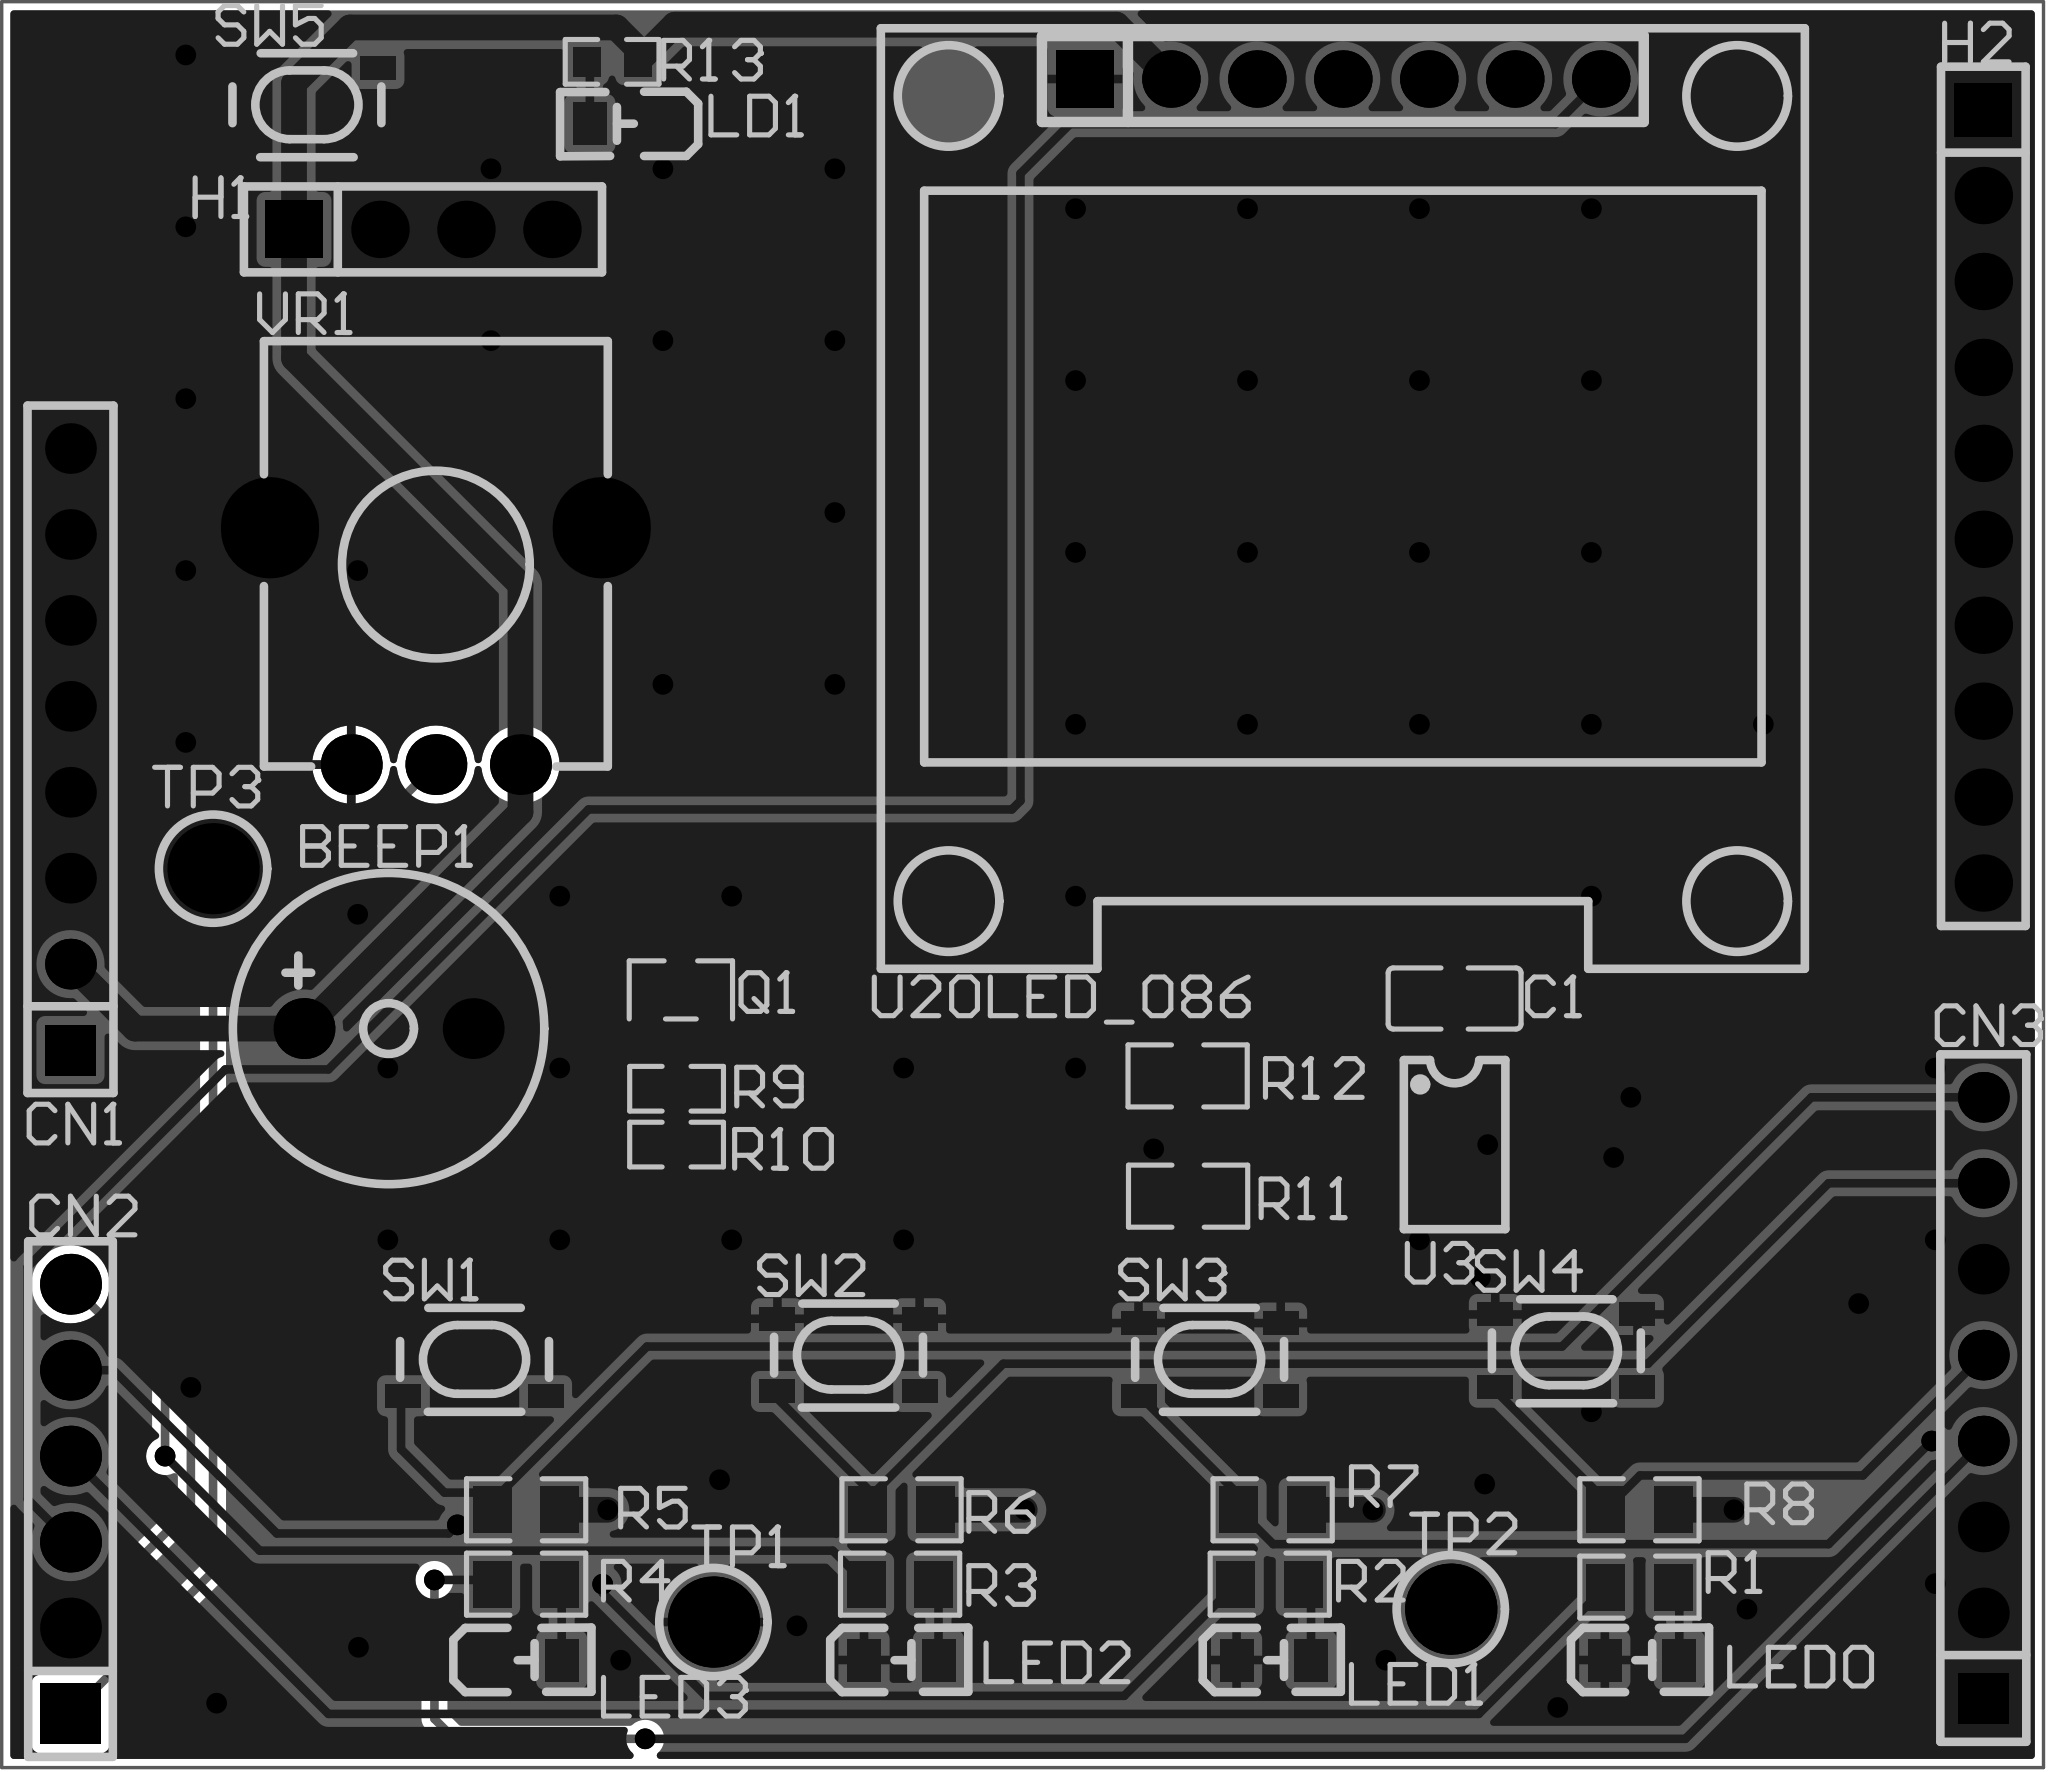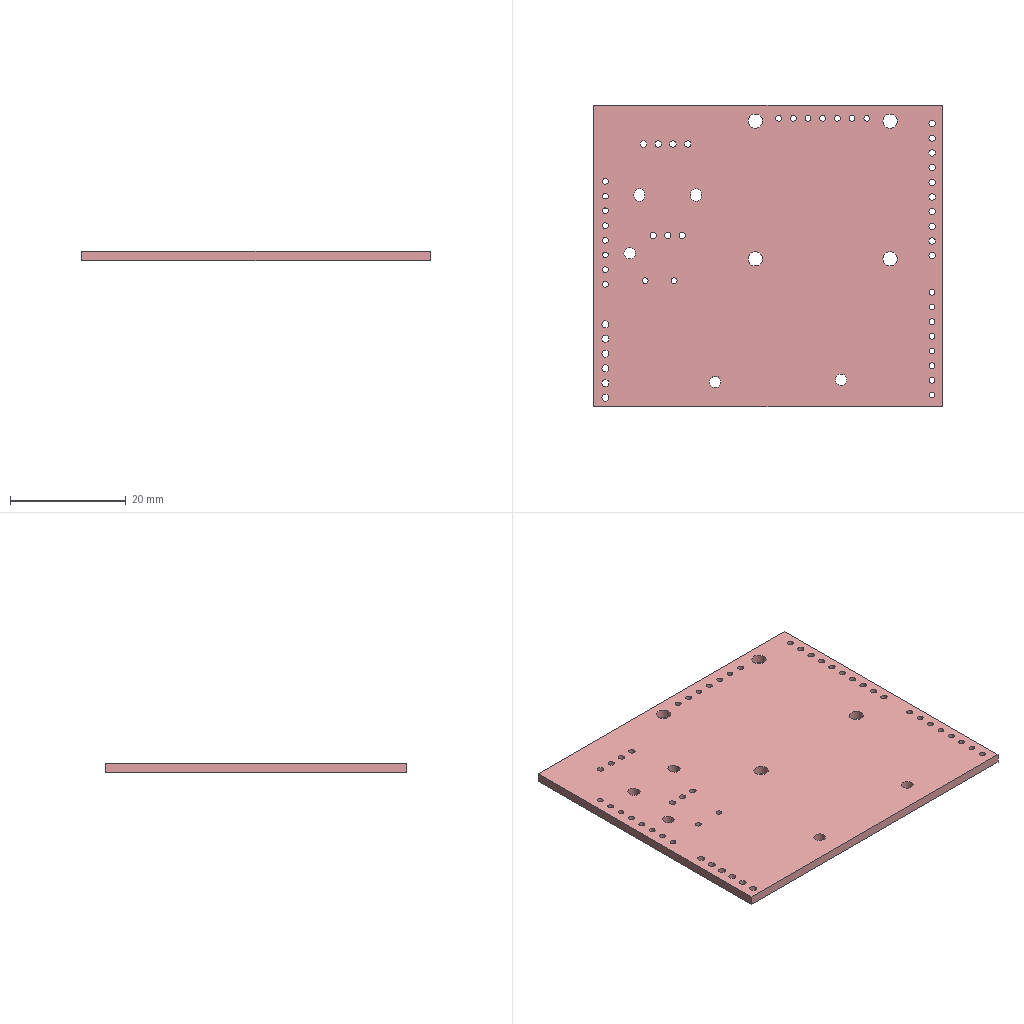Circuit board layout | Altium Designer | box 60.3 x 52.2 x 1.6 mm
Layer stack:
# Altium Designer layer stack of  (unit mm; dielectric type: 0 none, 1 core, 2 prepreg, 3 surface material)
index,name,kind,layer,copper_thickness_mm,dielectric_type,dielectric_thickness_mm,dielectric_material,dielectric_constant
0,Top Paste Mask Layer,other,,,,,,
1,Top Silkscreen Layer,other,,,,,,
2,Top Solder Mask Layer,dielectric,,,3,0.01,,3.3
3,Top Layer,copper,Top Layer,0.035,,,,
4,Dielectric1,dielectric,,,3,1.51,FR4,4.5
5,Bottom Layer,copper,Bottom Layer,0.035,,,,
6,Bottom Solder Mask Layer,dielectric,,,3,0.01,,3.3
7,Bottom Silkscreen Layer,other,,,,,,
8,Bottom Paste Mask Layer,other,,,,,,
# drill layer pairs: low layer,high layer
drill_pair,Top Layer,Bottom Layer
Part placement:
Designator,Comment,Layer,Footprint,Center-X(mm),Center-Y(mm),Rotation
BEEP1,3kHz,TopLayer,BUZ-TH_BD9.0-P5.00-D0.6-FD,96.139,112.014,0
C1,100nF,TopLayer,C0805,127.635,112.903,180
CN1,,TopLayer,HDR-TH_8P-P2.54-V-M,86.741,120.269,90
CN2,,TopLayer,HDR-TH_6P-P2.54-V-M-1,86.742,98.106,90
CN3,,TopLayer,HDR-TH_8P-P2.54-V-M,143.256,101.092,90
H1,,TopLayer,HDR-TH_4P-P2.54-V-F,97.155,135.636,0
H2,,TopLayer,HDR-TH_10P-P2.54-V-M-1,143.256,127.746,270
LD1,NCD0805R1,TopLayer,LED0805-RD,103.186,138.756,180
LED0,,TopLayer,LED_0805,133.173,93.35,0
LED1,,TopLayer,LED_0805,122.293,93.35,0
LED2,,TopLayer,LED_0805,111.287,93.35,0
LED3,,TopLayer,LED_0805,100.153,93.35,0
Q1,S8050 J3Y(RANGE:200-350),TopLayer,SOT-23-3_L3.0-W1.7-P0.95-LS2.9-BR,104.775,113.157,270
R1,4.7K,TopLayer,R0805,133.096,95.504,0
R2,4.7K,TopLayer,R0805,122.174,95.592,0
R3,4.7K,TopLayer,R0805,111.252,95.592,0
R4,4.7K,TopLayer,R0805,100.203,95.592,0
R5,4.7kΩ,TopLayer,R0805,100.203,97.79,0
R6,4.7kΩ,TopLayer,R0805,111.294,97.79,0
R7,4.7kΩ,TopLayer,R0805,122.259,97.79,0
R8,4.7kΩ,TopLayer,R0805,133.096,97.79,0
R9,1K,TopLayer,R0603,104.648,110.236,0
R10,10K,TopLayer,R0603,104.648,108.585,180
R11,4.7kΩ,TopLayer,R0805,119.761,107.061,180
R12,4.7kΩ,TopLayer,R0805,119.747,110.615,0
R13,4.7K,TopLayer,R0603,102.743,140.589,0
TP1,TP-红色测试点,TopLayer,TESTPOINT-TH_BD3.2,105.736,94.472,0
TP2,TP-红色测试点,TopLayer,TESTPOINT-TH_BD3.2,127.521,94.853,0
TP3,TP-红色测试点,TopLayer,TESTPOINT-TH_BD3.2,90.953,116.74,0
U2OLED_086,0.96寸OLED_7P,TopLayer,OLED-TH_HS96L01W4S03,124.333,140.081,0
U3,LM75AD,118,TopLayer,SOIC-8_L5.0-W4.0-P1.27-LS6.0-BL,127.635,108.585,270
VR1,10kΩ,TopLayer,RES-ADJ-TH_RK09K1130AJ3,97.536,123.317,0
SW1,,TopLayer,Key_SMD_4.2x3.2x2.5,98.679,102.235,0
SW2,,TopLayer,Key_SMD_4.2x3.2x2.5,109.728,102.362,0
SW3,,TopLayer,Key_SMD_4.2x3.2x2.5,120.396,102.235,0
SW4,,TopLayer,Key_SMD_4.2x3.2x2.5,130.937,102.489,0
SW5,,TopLayer,Key_SMD_4.2x3.2x2.5,93.726,139.319,0
Pad and via stacks:
# Altium Designer via and pad stacks of  (unit mm). Each distinct definition once, with the count of objects using it.
# via: kind,start_layer,end_layer,hole_mm,diameter_mm,mode(0 simple;1 top-mid-bottom;2 full stack),diameter_per_layer,count,example_net
# pad: kind,layer,hole_mm,hole_type(0 round;1 square;2 slot),plating,top_size,top_shape(1 round;2 rect;3 octagon;9 rounded rect),mid_size,bottom_size,mode,footprint,size_per_layer,count,example
pad,Multi-Layer,1,0,plated,1.8x1.8,1,1.8x1.8,1.8x1.8,0,BUZ-TH_BD9.0-P5.00-D0.6-FD,,2,BEEP1.1
pad,Multi-Layer,1,0,plated,1.5x1.5,2,1.5x1.5,1.5x1.5,0,HDR-TH_8P-P2.54-V-M,,2,CN1.1
pad,Multi-Layer,1,0,plated,1.5x1.5,1,1.5x1.5,1.5x1.5,0,HDR-TH_8P-P2.54-V-M,,14,CN1.2
pad,Multi-Layer,1.2,0,plated,1.8x1.8,1,1.8x1.8,1.8x1.8,0,HDR-TH_6P-P2.54-V-M-1,,5,CN2.6
pad,Multi-Layer,1.2,0,plated,1.8x1.8,2,1.8x1.8,1.8x1.8,0,HDR-TH_6P-P2.54-V-M-1,,1,CN2.1
pad,Multi-Layer,1.1,0,plated,1.7x1.7,2,1.7x1.7,1.7x1.7,0,HDR-TH_4P-P2.54-V-F,,1,H1.1
pad,Multi-Layer,1.1,0,plated,1.7x1.7,1,1.7x1.7,1.7x1.7,0,HDR-TH_4P-P2.54-V-F,,3,H1.2
pad,Multi-Layer,1.1,0,plated,1.7x1.7,1,1.7x1.7,1.7x1.7,0,HDR-TH_10P-P2.54-V-M-1,,9,H2.10
pad,Multi-Layer,1.1,0,plated,1.575x1.7,2,1.575x1.7,1.575x1.7,0,HDR-TH_10P-P2.54-V-M-1,,1,H2.1
pad,Multi-Layer,2,0,plated,2.7x2.7,1,2.7x2.7,2.7x2.7,0,TESTPOINT-TH_BD3.2,,3,TP1.1
pad,Multi-Layer,1,0,plated,1.7x1.7,1,1.7x1.7,1.7x1.7,0,OLED-TH_HS96L01W4S03,,6,U2OLED_086.7
pad,Multi-Layer,1,0,plated,1.7x1.7,2,1.7x1.7,1.7x1.7,0,OLED-TH_HS96L01W4S03,,1,U2OLED_086.1
pad,Multi-Layer,1.9,2,plated,2.9x3,1,2.9x3,2.9x3,0,RES-ADJ-TH_RK09K1130AJ3,,2,VR1.5
pad,Multi-Layer,1.1,0,plated,1.8x1.8,1,1.8x1.8,1.8x1.8,0,RES-ADJ-TH_RK09K1130AJ3,,3,VR1.3
pad,Top Layer,0,0,plated,1.41x1.35,2,1.41x1.35,1.41x1.35,0,C0805,,2,C1.2
pad,Top Layer,0,0,plated,1x1.25,2,1x1.25,1x1.25,0,LED0805-RD,,2,LD1.2
pad,Top Layer,0,0,plated,1x1.25,2,1x1.25,1x1.25,0,LED_0805,,8,LED0.2
pad,Top Layer,0,0,plated,1.038x0.532,2,1.038x0.532,1.038x0.532,0,SOT-23-3_L3.0-W1.7-P0.95-LS2.9-BR,,3,Q1.1
pad,Top Layer,0,0,plated,1.133x1.377,2,1.133x1.377,1.133x1.377,0,R0805,,20,R1.2
pad,Top Layer,0,0,plated,0.8065x0.864,2,0.8065x0.864,0.8065x0.864,0,R0603,,6,R9.2
pad,Top Layer,0,0,plated,0.5684x1.95,1,0.5684x1.95,0.5684x1.95,0,SOIC-8_L5.0-W4.0-P1.27-LS6.0-BL,,8,U3.1
pad,Top Layer,0,0,plated,1.049x0.701,2,1.049x0.701,1.049x0.701,0,Key_SMD_4.2x3.2x2.5,,20,SW1.1
via,Top Layer,Bottom Layer,0.3048,0.61,0,,76,PB4
Copper pours:
name,layer,net,type(0 solid;1 hatched;2 none)
Bottom Layer-GND,Bottom Layer,GND,0
Top Layer-GND,Top Layer,GND,0